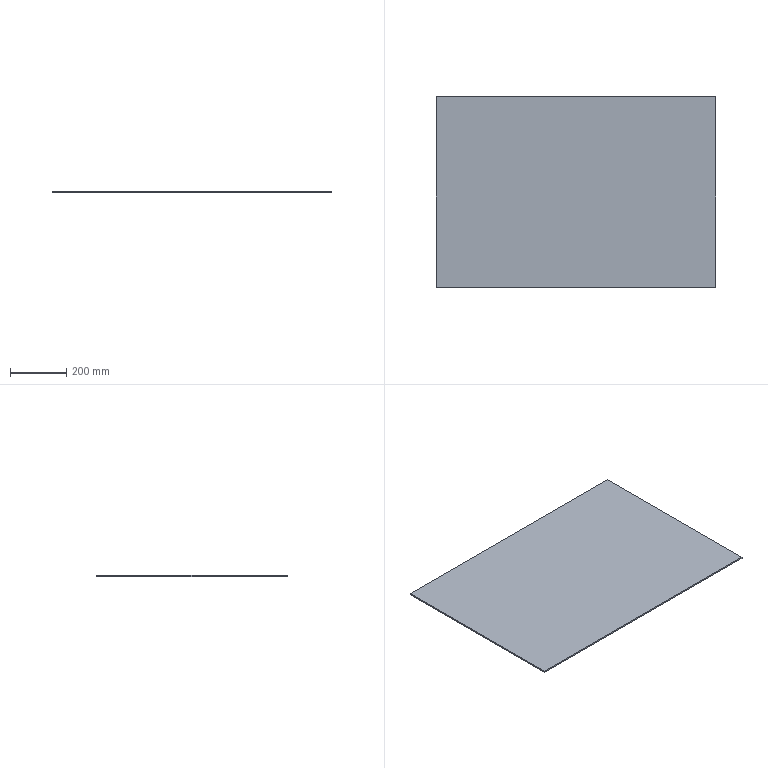Part | SolidWorks | features Extrusion 1 | 1 solid | 6 faces | box 997 x 678 x 5 mm | volume 3379830 mm3 | plane 6
STEP:
#1=CARTESIAN_POINT('',(498.5,-339.,0.));
#2=VERTEX_POINT('',#1);
#3=CARTESIAN_POINT('',(498.5,339.,0.));
#4=VERTEX_POINT('',#3);
#5=CARTESIAN_POINT('',(498.5,339.,0.));
#6=DIRECTION('',(0.,1.,0.));
#7=VECTOR('',#6,1000.);
#8=LINE('',#5,#7);
#9=EDGE_CURVE('',#2,#4,#8,.T.);
#10=ORIENTED_EDGE('',*,*,#9,.T.);
#11=CARTESIAN_POINT('',(498.5,339.,5.));
#12=VERTEX_POINT('',#11);
#13=CARTESIAN_POINT('',(498.5,339.,5.));
#14=DIRECTION('',(0.,0.,-1.));
#15=VECTOR('',#14,1000.);
#16=LINE('',#13,#15);
#17=EDGE_CURVE('',#12,#4,#16,.T.);
#18=ORIENTED_EDGE('',*,*,#17,.F.);
#19=CARTESIAN_POINT('',(498.5,-339.,5.));
#20=VERTEX_POINT('',#19);
#21=CARTESIAN_POINT('',(498.5,339.,5.));
#22=DIRECTION('',(0.,1.,0.));
#23=VECTOR('',#22,1000.);
#24=LINE('',#21,#23);
#25=EDGE_CURVE('',#20,#12,#24,.T.);
#26=ORIENTED_EDGE('',*,*,#25,.F.);
#27=CARTESIAN_POINT('',(498.5,-339.,5.));
#28=DIRECTION('',(0.,0.,-1.));
#29=VECTOR('',#28,1000.);
#30=LINE('',#27,#29);
#31=EDGE_CURVE('',#20,#2,#30,.T.);
#32=ORIENTED_EDGE('',*,*,#31,.T.);
#33=EDGE_LOOP('',(#10,#18,#26,#32));
#34=FACE_OUTER_BOUND('',#33,.T.);
#35=CARTESIAN_POINT('',(498.5,339.,5.));
#36=DIRECTION('',(-1.,0.,0.));
#37=DIRECTION('',(0.,-1.,0.));
#38=AXIS2_PLACEMENT_3D('',#35,#36,#37);
#39=PLANE('',#38);
#40=ADVANCED_FACE('',(#34),#39,.F.);
#41=CARTESIAN_POINT('',(-498.5,339.,0.));
#42=VERTEX_POINT('',#41);
#43=CARTESIAN_POINT('',(-498.5,339.,0.));
#44=DIRECTION('',(-1.,0.,0.));
#45=VECTOR('',#44,1000.);
#46=LINE('',#43,#45);
#47=EDGE_CURVE('',#4,#42,#46,.T.);
#48=ORIENTED_EDGE('',*,*,#47,.T.);
#49=CARTESIAN_POINT('',(-498.5,339.,5.));
#50=VERTEX_POINT('',#49);
#51=CARTESIAN_POINT('',(-498.5,339.,5.));
#52=DIRECTION('',(0.,0.,-1.));
#53=VECTOR('',#52,1000.);
#54=LINE('',#51,#53);
#55=EDGE_CURVE('',#50,#42,#54,.T.);
#56=ORIENTED_EDGE('',*,*,#55,.F.);
#57=CARTESIAN_POINT('',(-498.5,339.,5.));
#58=DIRECTION('',(-1.,0.,0.));
#59=VECTOR('',#58,1000.);
#60=LINE('',#57,#59);
#61=EDGE_CURVE('',#12,#50,#60,.T.);
#62=ORIENTED_EDGE('',*,*,#61,.F.);
#63=ORIENTED_EDGE('',*,*,#17,.T.);
#64=EDGE_LOOP('',(#48,#56,#62,#63));
#65=FACE_OUTER_BOUND('',#64,.T.);
#66=CARTESIAN_POINT('',(-498.5,339.,5.));
#67=DIRECTION('',(0.,-1.,0.));
#68=DIRECTION('',(0.,0.,-1.));
#69=AXIS2_PLACEMENT_3D('',#66,#67,#68);
#70=PLANE('',#69);
#71=ADVANCED_FACE('',(#65),#70,.F.);
#72=CARTESIAN_POINT('',(-498.5,-339.,0.));
#73=VERTEX_POINT('',#72);
#74=CARTESIAN_POINT('',(-498.5,339.,0.));
#75=DIRECTION('',(0.,-1.,0.));
#76=VECTOR('',#75,1000.);
#77=LINE('',#74,#76);
#78=EDGE_CURVE('',#42,#73,#77,.T.);
#79=ORIENTED_EDGE('',*,*,#78,.T.);
#80=CARTESIAN_POINT('',(-498.5,-339.,5.));
#81=VERTEX_POINT('',#80);
#82=CARTESIAN_POINT('',(-498.5,-339.,5.));
#83=DIRECTION('',(0.,0.,-1.));
#84=VECTOR('',#83,1000.);
#85=LINE('',#82,#84);
#86=EDGE_CURVE('',#81,#73,#85,.T.);
#87=ORIENTED_EDGE('',*,*,#86,.F.);
#88=CARTESIAN_POINT('',(-498.5,339.,5.));
#89=DIRECTION('',(0.,-1.,0.));
#90=VECTOR('',#89,1000.);
#91=LINE('',#88,#90);
#92=EDGE_CURVE('',#50,#81,#91,.T.);
#93=ORIENTED_EDGE('',*,*,#92,.F.);
#94=ORIENTED_EDGE('',*,*,#55,.T.);
#95=EDGE_LOOP('',(#79,#87,#93,#94));
#96=FACE_OUTER_BOUND('',#95,.T.);
#97=CARTESIAN_POINT('',(-498.5,339.,5.));
#98=DIRECTION('',(1.,0.,0.));
#99=DIRECTION('',(0.,1.,0.));
#100=AXIS2_PLACEMENT_3D('',#97,#98,#99);
#101=PLANE('',#100);
#102=ADVANCED_FACE('',(#96),#101,.F.);
#103=CARTESIAN_POINT('',(-498.5,-339.,0.));
#104=DIRECTION('',(1.,0.,0.));
#105=VECTOR('',#104,1000.);
#106=LINE('',#103,#105);
#107=EDGE_CURVE('',#73,#2,#106,.T.);
#108=ORIENTED_EDGE('',*,*,#107,.T.);
#109=ORIENTED_EDGE('',*,*,#31,.F.);
#110=CARTESIAN_POINT('',(-498.5,-339.,5.));
#111=DIRECTION('',(1.,0.,0.));
#112=VECTOR('',#111,1000.);
#113=LINE('',#110,#112);
#114=EDGE_CURVE('',#81,#20,#113,.T.);
#115=ORIENTED_EDGE('',*,*,#114,.F.);
#116=ORIENTED_EDGE('',*,*,#86,.T.);
#117=EDGE_LOOP('',(#108,#109,#115,#116));
#118=FACE_OUTER_BOUND('',#117,.T.);
#119=CARTESIAN_POINT('',(-498.5,-339.,5.));
#120=DIRECTION('',(0.,1.,0.));
#121=DIRECTION('',(0.,0.,1.));
#122=AXIS2_PLACEMENT_3D('',#119,#120,#121);
#123=PLANE('',#122);
#124=ADVANCED_FACE('',(#118),#123,.F.);
#125=ORIENTED_EDGE('',*,*,#25,.T.);
#126=ORIENTED_EDGE('',*,*,#61,.T.);
#127=ORIENTED_EDGE('',*,*,#92,.T.);
#128=ORIENTED_EDGE('',*,*,#114,.T.);
#129=EDGE_LOOP('',(#125,#126,#127,#128));
#130=FACE_OUTER_BOUND('',#129,.T.);
#131=CARTESIAN_POINT('',(0.,0.,5.));
#132=DIRECTION('',(0.,0.,1.));
#133=DIRECTION('',(1.,0.,0.));
#134=AXIS2_PLACEMENT_3D('',#131,#132,#133);
#135=PLANE('',#134);
#136=ADVANCED_FACE('',(#130),#135,.T.);
#137=ORIENTED_EDGE('',*,*,#9,.F.);
#138=ORIENTED_EDGE('',*,*,#107,.F.);
#139=ORIENTED_EDGE('',*,*,#78,.F.);
#140=ORIENTED_EDGE('',*,*,#47,.F.);
#141=EDGE_LOOP('',(#137,#138,#139,#140));
#142=FACE_OUTER_BOUND('',#141,.T.);
#143=CARTESIAN_POINT('',(0.,0.,0.));
#144=DIRECTION('',(0.,0.,1.));
#145=DIRECTION('',(1.,0.,0.));
#146=AXIS2_PLACEMENT_3D('',#143,#144,#145);
#147=PLANE('',#146);
#148=ADVANCED_FACE('',(#142),#147,.F.);
#149=CLOSED_SHELL('',(#40,#71,#102,#124,#136,#148));
#150=MANIFOLD_SOLID_BREP('',#149);
#151=CARTESIAN_POINT('',(0.,0.,0.));
#152=DIRECTION('',(0.,0.,1.));
#153=DIRECTION('',(1.,0.,0.));
#154=AXIS2_PLACEMENT_3D('',#151,#152,#153);
#155=(LENGTH_UNIT()NAMED_UNIT(*)SI_UNIT(.MILLI.,.METRE.));
#156=UNCERTAINTY_MEASURE_WITH_UNIT(LENGTH_MEASURE(0.00001),#155,'','');
#157=(NAMED_UNIT(*)PLANE_ANGLE_UNIT()SI_UNIT($,.RADIAN.));
#158=(NAMED_UNIT(*)SI_UNIT($,.STERADIAN.)SOLID_ANGLE_UNIT());
#159=(GEOMETRIC_REPRESENTATION_CONTEXT(3)GLOBAL_UNCERTAINTY_ASSIGNED_CONTEXT((#156))GLOBAL_UNIT_ASSIGNED_CONTEXT((#155,#157,#158))REPRESENTATION_CONTEXT('',''));
#160=ADVANCED_BREP_SHAPE_REPRESENTATION('',(#150,#154),#159);